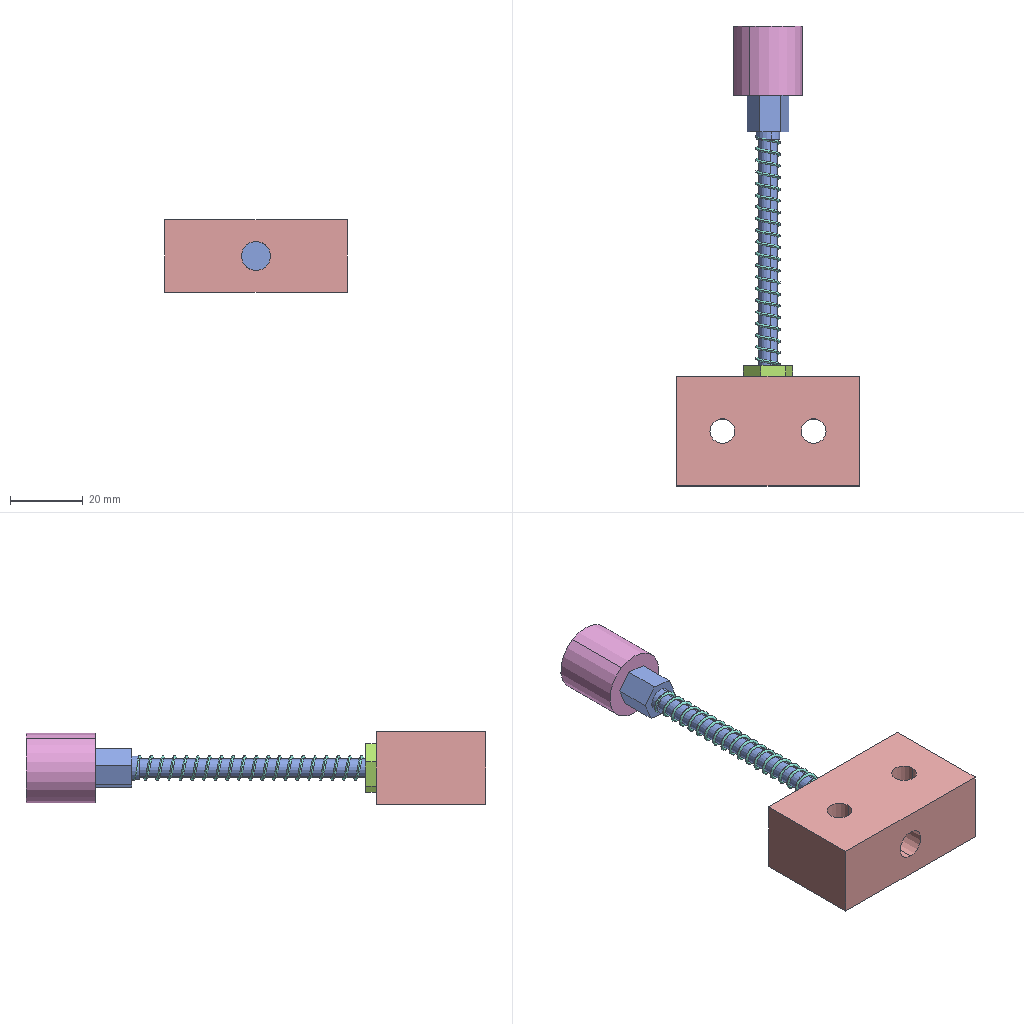Assembly | SolidWorks | 4 different items | 4 placed | box 50 x 126 x 20 mm
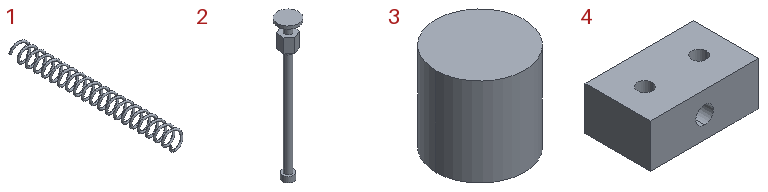Parts list (item | quantity | size | volume | features):
1 | x1 | 6.8 x 64.8 x 6.8 mm | 188.36 mm3 | features Sweep 1
2 | x1 | 15 x 15 x 100 mm | 3078 mm3 | features ICE 5, Extrusion 1
3 | x1 | 19 x 19 x 19 mm | 5387 mm3 | features Extrusion 1
4 | x1 | 50 x 30 x 20 mm | 27179 mm3 | features HoleWzd 2, 3DProfileFeature 1, Extrusion 1, ICE 1
Mates (type | each side: item.copy, entity, surface, feature):
Concentric | 2.1 face cylinder Boss-Extrude3 | 3.1 face cylinder Boss-Extrude1
DistanceDim | 2.1 face plane Boss-Extrude3 | 3.1 face plane Boss-Extrude1
Concentric | 2.1 face cylinder Boss-Extrude1 | 1.1 select_type:24